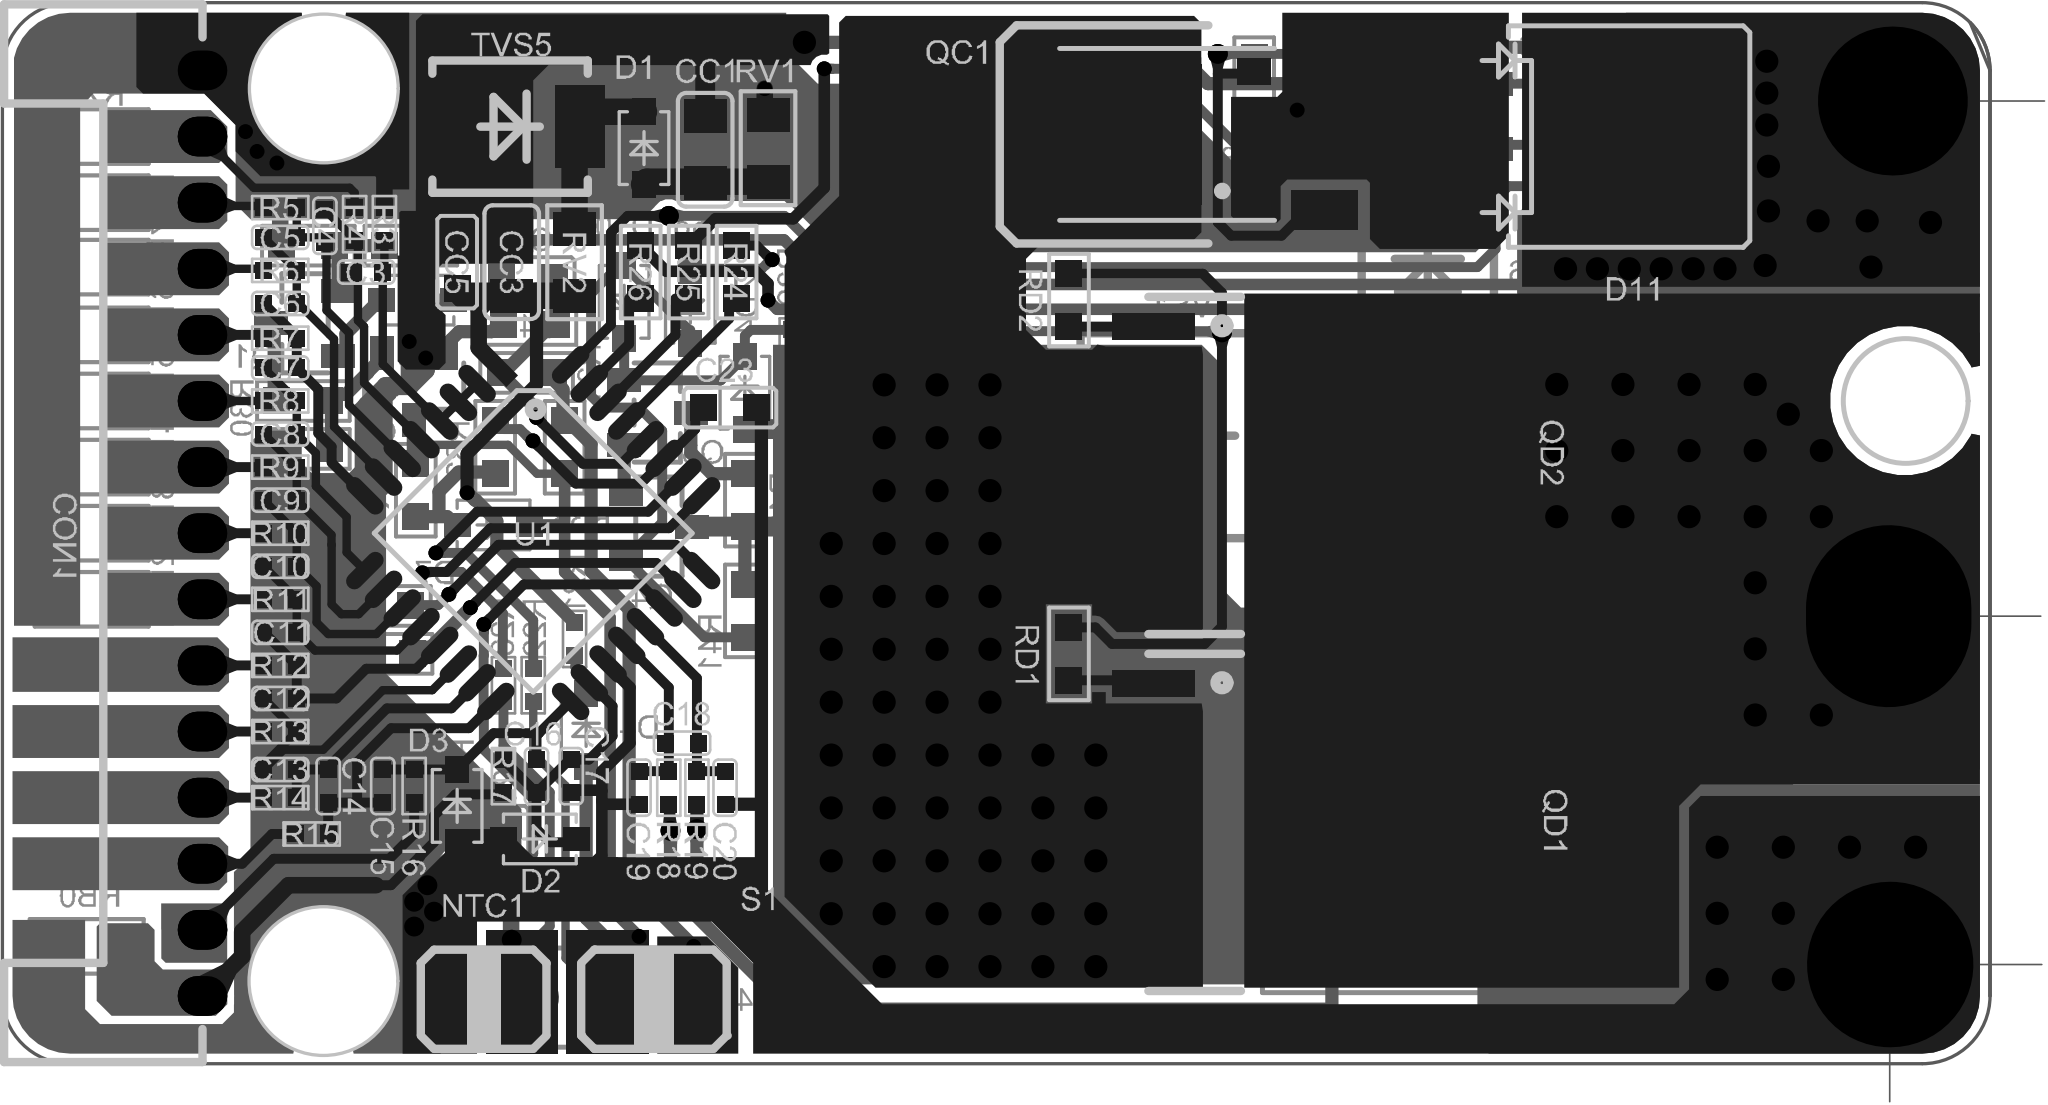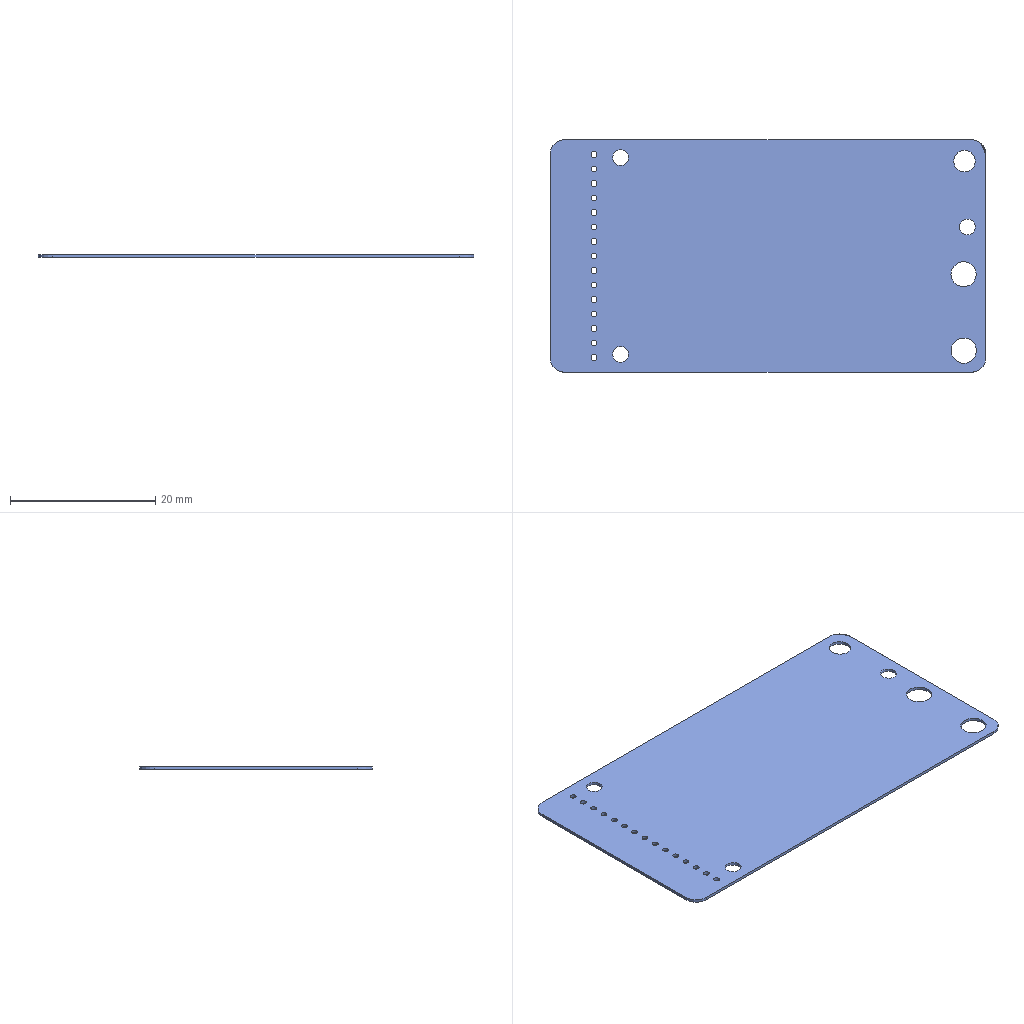Circuit board layout | Altium Designer | box 60.1 x 32.1 x 0.4 mm
Layer stack:
# Altium Designer layer stack of  (unit mm; dielectric type: 0 none, 1 core, 2 prepreg, 3 surface material)
index,name,kind,layer,copper_thickness_mm,dielectric_type,dielectric_thickness_mm,dielectric_material,dielectric_constant
0,Top Paste,other,,,,,,
1,Top Overlay,other,,,,,,
2,Top Solder,dielectric,,,3,0.0102,Solder Resist,3.5
3,Top Layer,copper,Top Layer,0.0356,,,,
4,Dielectric 1,dielectric,,,0,0.32,FR-4,4.8
5,Bottom Layer,copper,Bottom Layer,0.0356,,,,
6,Bottom Solder,dielectric,,,3,0.0102,Solder Resist,3.5
7,Bottom Overlay,other,,,,,,
8,Bottom Paste,other,,,,,,
# drill layer pairs: low layer,high layer
drill_pair,Top Layer,Bottom Layer
Part placement:
Designator,Comment,Layer,Footprint,Center-X(mm),Center-Y(mm),Rotation
D7,1N4148SW,BottomLayer,SOD323,14.8,0.25,180
ZD4,15V,BottomLayer,SOD323(1+2-),22.4,4.25,270
C1,0.1uF,BottomLayer,C0603A,15.85,7.75,180
QC1,NMOS,TopLayer,TO-252-DFN,35.416,12.065,0
RS3,R005,BottomLayer,R2512L,42.4,-12.05,180
RS2,R005,BottomLayer,R2512L,42.4,-7.95,180
RS1,R005,BottomLayer,R2512L,42.4,-3.85,180
TVS5,SMBJ64A,TopLayer,SMB_M(1+2-),15.3,12.3,180
D1,BAV21W,TopLayer,SOD323(1+2-),19.35,11.65,270
RX8,0Ω,BottomLayer,R0805L,2.65,12,0
RX7,0Ω,BottomLayer,R0805L,2.65,10,0
RX6,0Ω,BottomLayer,R0805L,2.65,8.05,0
RX5,0Ω,BottomLayer,R0805L,2.65,6,0
RX4,0Ω,BottomLayer,R0805L,2.65,4,0
RX3,0Ω,BottomLayer,R0805L,2.65,2,0
RX2,0Ω,BottomLayer,R0805L,2.65,0,0
RX1,0Ω,BottomLayer,R0805L,2.65,-2,0
RV2,100Ω,TopLayer,R0805L,17.25,8.2,90
RV1,1KΩ,TopLayer,R0805L,23.1,11.65,90
CC5,100nF/100V,TopLayer,C0603A,13.7,8.2,270
CC3,1uF/100V,TopLayer,C0805L,15.35,8.2,270
CC1,1uF/100V,TopLayer,C0805L,21.2,11.6,270
J4,UART,BottomLayer,CH-2.0-4P,17,-14.05,180
D2,BAT46WS,TopLayer,SOD323(1+2-),16.2,-9.25,180
NTC1,10KNTC,TopLayer,RT2.3X1-2,14.5,-14.1,180
D11,MBR10100DCT,TopLayer,TO-252-DIODE-DUAL,46.388,12,270
S1,SW-SPST,TopLayer,RT2.3X1.2-2,19.65,-14.1,0
RX,0R,BottomLayer,R0603A,12.45,1.3,270
R45,10M,BottomLayer,R0603A,15.9,6.3,180
R34,100K,BottomLayer,R0603A,15.8,4.85,180
R33,0Ω/NC,BottomLayer,R0603A,16.95,2.6,270
R32,100K,BottomLayer,R0603A,14.85,2.6,270
R31,100K,BottomLayer,R0603A,9.05,2.55,0
R30,1M,BottomLayer,R0603A,9.05,4,180
R29,100K,BottomLayer,R0603A,12.3,8.7,180
R28,20K,BottomLayer,R0603A,9.2,8.7,180
Q2,MMBT5551,BottomLayer,SOT23-3_BEC,12.4,4.442,0
Q1,MMBT5401,BottomLayer,SOT23-3_BEC,9.092,6.35,270
C14,0.1uF,TopLayer,C0402A,9.8,-7.65,90
R9,510R,TopLayer,R0402A,8.35,2,180
R8,510R,TopLayer,R0402A,8.35,4,180
R10,510R,TopLayer,R0402A,8.35,0,180
R13,510R,TopLayer,R0402A,8.35,-6,180
R12,510R,TopLayer,R0402A,8.35,-4,180
R11,510R,TopLayer,R0402A,8.35,-2,180
CON1,Header 15,TopLayer,PH-2.0mm15P弯脚不带扣,6,0,90
ZD2,15V,BottomLayer,SOD323(1+2-),12.5,7.05,180
ZD1,15V,BottomLayer,SOD323(1+2-),39.5,13.4,270
U1,SH3676016B,TopLayer,LQFP32L(PIN间距0.8mm),16,0,315
TVS1,75CA,BottomLayer,SMC,36.1,2.95,0
RTX,NC,BottomLayer,R0603A,13.8,-9.65,90
RT3,10K,BottomLayer,R0603A,11.5,-2.2,180
RT2,10K,BottomLayer,R0603A,11.55,-3.65,180
RD2,47R,TopLayer,R0603Ap,32.2,7.05,270
RD1,47R,TopLayer,R0603Ap,32.2,-3.65,270
RB0,51R,BottomLayer,R0805L,2.5,-12.5,0
R41,4.7M,BottomLayer,R0603A,22.4,-2.35,270
R40,510R,BottomLayer,R0603A,22.4,1,270
R39,10M,BottomLayer,R0402A,23.8,5.65,90
R38,1M,BottomLayer,R0603A,37.8,13.6,90
R37,3M,BottomLayer,R0603A,48.25,12.8,90
R36,1M,BottomLayer,R0603A,46.7,12.8,270
R27,3M,BottomLayer,R0603A,47.4,10.5,180
R26,1M,TopLayer,R0603A,19.25,7.9,270
R25,1K,TopLayer,R0603A,20.7,7.9,270
R24,1K,TopLayer,R0603A,22.15,7.9,270
R23,100R,BottomLayer,R0402A,15.1,-4.6,90
R22,100R,BottomLayer,R0402A,16,-4.6,90
R21,100R,BottomLayer,R0402A,17.25,-3.2,90
R19,10R,TopLayer,R0402A,20.95,-7.7,270
R18,10R,TopLayer,R0402A,20.1,-7.7,270
R17,510R,TopLayer,R0402A,15.1,-7.35,270
R16,510R,TopLayer,R0402A,12.4,-7.65,270
R15,510R,TopLayer,R0402A,9.3,-9.1,0
R14,510R,TopLayer,R0402A,8.35,-8,180
R7,510R,TopLayer,R0402A,8.35,5.9,180
R6,510R,TopLayer,R0402A,8.35,7.95,180
R5,510R,TopLayer,R0402A,8.35,9.85,180
R4,510R,TopLayer,R0402A,10.6,9.35,90
R3,510R,TopLayer,R0402A,11.5,9.35,90
QD2,NMOS,TopLayer,TOLL,38.15,2.05,270
QD1,NMOS,TopLayer,TOLL,38.15,-8.75,270
Q5,MMBT5401,BottomLayer,SOT23-3,44.092,12.6,270
Q4,MMBT5401,BottomLayer,SOT23-3,19.808,0.2,90
Q3,MMBT5401,BottomLayer,SOT23-3,19.758,3.65,90
D10,BAV21WS,BottomLayer,SOD323(1+2-),18.75,7,90
D9,BAV21WS,BottomLayer,SOD323(1+2-),20.75,6.85,90
D6,RS3M,BottomLayer,SMB_M(1+2-),43.05,7.8,270
D5,BAV21WS,BottomLayer,SOD323(1+2-),41.4,13.4,270
D4,BAV21WS,BottomLayer,SOD323(1+2-),17.6,-5.95,270
D3,BAT46WS,TopLayer,SOD323(1+2-),13.7,-8.25,270
C23,1uF/25V,TopLayer,C0603A,21.95,3.8,180
C21,1000PF,BottomLayer,C0603A,15.25,-9.65,90
C20,1uF,TopLayer,C0402A,21.8,-7.7,270
C19,1uF,TopLayer,C0402A,19.2,-7.7,270
C18,1000PF,TopLayer,C0402A,20.5,-6.35,180
C17,1uF,TopLayer,C0402A,17.15,-7.35,90
C16,0.1uF,TopLayer,C0402A,16.1,-7.35,90
C15,0.1uF,TopLayer,C0402A,11.45,-7.65,270
C13,0.1uF,TopLayer,C0402A,8.35,-7.15,180
C12,0.1uF,TopLayer,C0402A,8.35,-5,0
C11,0.1uF,TopLayer,C0402A,8.35,-3,0
C10,0.1uF,TopLayer,C0402A,8.35,-1,0
C9,0.1uF,TopLayer,C0402A,8.35,1,0
C8,0.1uF,TopLayer,C0402A,8.35,3,0
C7,0.1uF,TopLayer,C0402A,8.35,5,0
C6,0.1uF,TopLayer,C0402A,8.35,6.95,0
C5,0.1uF,TopLayer,C0402A,8.35,8.95,0
C4,0.1uF,TopLayer,C0402A,9.7,9.3,90
C3,0.1uF,TopLayer,C0402A,10.95,7.9,0
Pad and via stacks:
# Altium Designer via and pad stacks of  (unit mm). Each distinct definition once, with the count of objects using it.
# via: kind,start_layer,end_layer,hole_mm,diameter_mm,mode(0 simple;1 top-mid-bottom;2 full stack),diameter_per_layer,count,example_net
# pad: kind,layer,hole_mm,hole_type(0 round;1 square;2 slot),plating,top_size,top_shape(1 round;2 rect;3 octagon;9 rounded rect),mid_size,bottom_size,mode,footprint,size_per_layer,count,example
pad,Keep-Out Layer,0.025,0,plated,0.025x0.025,1,0.025x0.025,0.025x0.025,0,,,2,1
pad,Bottom Layer,0,0,plated,0.8x0.7,2,0.8x0.7,0.8x0.7,0,SOD323,,2,D7.2
pad,Bottom Layer,0,0,plated,0.8x0.8,2,0.8x0.8,0.8x0.8,0,R0603A,,36,R33.1
pad,Bottom Layer,0,0,plated,0.5x0.5,2,0.5x0.5,0.5x0.5,0,R0402A,,8,R39.2
pad,Bottom Layer,0,0,plated,2x3.2,2,2x3.2,2x3.2,0,R2512L,,6,RS2.1
pad,Bottom Layer,0,0,plated,1.016x1.27,2,1.016x1.27,1.016x1.27,0,R0805L,,18,RX8.1
pad,Bottom Layer,0,0,plated,0.8x0.7,2,0.8x0.7,0.8x0.7,0,SOD323(1+2-),,14,ZD4.1
pad,Bottom Layer,0,0,plated,0.8x0.8,2,0.8x0.8,0.8x0.8,0,C0603A,,4,C21.1
pad,Bottom Layer,0,0,plated,1.5x1.5,2,1.5x1.5,1.5x1.5,0,CH-2.0-4P,,1,J4.1
pad,Bottom Layer,0,0,plated,1.5x1.5,1,1.5x1.5,1.5x1.5,0,CH-2.0-4P,,3,J4.2
pad,Bottom Layer,0,0,plated,0.7x1,2,0.7x1,0.7x1,0,SOT23-3_BEC,,6,Q2.B
pad,Bottom Layer,0,0,plated,0.7x1,2,0.7x1,0.7x1,0,SOT23-3,,9,Q3.3
pad,Bottom Layer,0,0,plated,1.5x2.5,2,1.5x2.5,1.5x2.5,0,SMB M(1+2-),,2,D6.2
pad,Bottom Layer,0,0,plated,2.44x3.62,2,2.44x3.62,2.44x3.62,0,SMC,,2,TVS1.1
pad,Top Layer,0,0,plated,0.8x0.8,2,0.8x0.8,0.8x0.8,0,C0603A,,4,CC5.2
pad,Top Layer,0,0,plated,0.8x0.8,2,0.8x0.8,0.8x0.8,0,R0603A,,6,R24.2
pad,Top Layer,0,0,plated,0.5x0.5,2,0.5x0.5,0.5x0.5,0,C0402A,,36,C20.1
pad,Top Layer,0,0,plated,0.5x0.5,2,0.5x0.5,0.5x0.5,0,R0402A,,34,R19.2
pad,Top Layer,0,0,plated,2.5x0.8,2,2.5x0.8,2.5x0.8,0,TOLL,,2,QD2.1
pad,Top Layer,0,0,plated,1.7x0.8,2,1.7x0.8,1.7x0.8,0,TOLL,,14,QD2.2
pad,Top Layer,0,0,plated,0.8x8,2,0.8x8,0.8x8,0,TOLL,,2,QD2.2
pad,Top Layer,0,0,plated,9.9x8,2,9.9x8,9.9x8,0,TOLL,,2,QD2.3
pad,Top Layer,0,0,plated,3x4.26,2,3x4.26,3x4.26,0,TO-252-DFN,,1,QC1.3
pad,Top Layer,0,0,plated,1x0.8,2,1x0.8,1x0.8,0,TO-252-DFN,,8,QC1.2
pad,Top Layer,0,0,plated,1.2x2,2,1.2x2,1.2x2,0,TO-252-DFN,,2,QC1.1
pad,Top Layer,0,0,plated,5.3x1,2,5.3x1,5.3x1,0,TO-252-DFN,,1,QC1.3
pad,Top Layer,0,0,plated,6x6,2,6x6,6x6,0,TO-252-DIODE-DUAL,,1,D11.3
pad,Top Layer,0,0,plated,1.3x2.5,2,1.3x2.5,1.3x2.5,0,TO-252-DIODE-DUAL,,2,D11.2
pad,Top Layer,0,0,plated,0.8x0.8,2,0.8x0.8,0.8x0.8,0,R0603Ap,,4,RD1.1
pad,Top Layer,0,0,plated,1.016x1.27,2,1.016x1.27,1.016x1.27,0,R0805L,,4,RV2.2
pad,Top Layer,0,0,plated,1.5x2.5,2,1.5x2.5,1.5x2.5,0,SMB M(1+2-),,2,TVS5.2
pad,Top Layer,0,0,plated,1.016x1.27,2,1.016x1.27,1.016x1.27,0,C0805L,,4,CC1.1
pad,Top Layer,0,0,plated,1.2x2.3,1,1.2x2.3,1.2x2.3,0,RT2.3X1.2-2,,2,S1.1
pad,Top Layer,0,0,plated,1x2.3,1,1x2.3,1x2.3,0,RT2.3X1-2,,2,NTC1.1
pad,Top Layer,0,0,plated,0.8x0.7,2,0.8x0.7,0.8x0.7,0,SOD323(1+2-),,6,D2.1
pad,Top Layer,0,0,plated,0.5x1.4,1,0.5x1.4,0.5x1.4,0,LQFP32L(PIN\u00BC\u00E4\u00BE\u00E00.8mm),,31,U1.29
pad,Top Layer,0,0,plated,0.5x1.4,2,0.5x1.4,0.5x1.4,0,LQFP32L(PIN\u00BC\u00E4\u00BE\u00E00.8mm),,1,U1.1
pad,Multi-Layer,0.8,0,plated,1.5x1.2,1,1.5x1.2,1.5x1.2,0,PH-2.0mm15P\u00CD\u00E4\u00BD\u00C5\u00B2\u00BB\u00B4\u00F8\u00BF\u00DB,,15,CON1.11
pad,Multi-Layer,3.5,0,plated,5x5.5,1,5x5.5,5x5.5,0,,,1,2
pad,Multi-Layer,3,0,plated,4.5x4.5,1,4.5x4.5,4.5x4.5,0,,,1,2
pad,Multi-Layer,3.5,0,plated,5x5,1,5x5,5x5,0,,,1,2
pad,Top Solder,0,0,plated,12x2.5,2,12x2.5,12x2.5,0,,,1,2
pad,Top Solder,0,0,plated,20x2.5,2,20x2.5,20x2.5,0,,,1,2
pad,Top Solder,0,0,plated,15x2.5,2,15x2.5,15x2.5,0,,,2,2
pad,Bottom Solder,0,0,plated,15x2.5,2,15x2.5,15x2.5,0,,,2,2
via,Top Layer,Bottom Layer,0.3,0.45,0,,20,VCC1
via,Top Layer,Bottom Layer,0.4,0.6,0,,10,NetR27_2
via,Top Layer,Bottom Layer,0.5,0.7,0,,98,RS2
Copper pours:
name,layer,net,type(0 solid;1 hatched;2 none)
NONET_L-01_P-001,Bottom Layer,B+,0
RS2_L02_P042,Bottom Layer,RS2,0
P-_L02_P041,Bottom Layer,P-,0
NONET_L-01_P-001,Bottom Layer,B-,0
NONET_L-01_P-001,Bottom Layer,B0,0
NONET_L-01_P-001,Bottom Layer,B1,0
NONET_L-01_P-001,Bottom Layer,B2,0
NONET_L-01_P-001,Bottom Layer,B3,0
NONET_L-01_P-001,Bottom Layer,B4,0
NONET_L-01_P-001,Bottom Layer,B5,0
C-_L02_P032,Bottom Layer,C-,0
NONET_L-01_P-001,Bottom Layer,B12,0
NONET_L-01_P-001,Bottom Layer,B13,0
NONET_L-01_P-001,Bottom Layer,B6,0
NONET_L-01_P-001,Bottom Layer,B7,0
NONET_L-01_P-001,Bottom Layer,B8,0
NONET_L-01_P-001,Bottom Layer,B9,0
NONET_L-01_P-001,Bottom Layer,B10,0
NONET_L-01_P-001,Bottom Layer,B11,0
NONET_L-01_P-001,Bottom Layer,B-,0
RS2_L01_P029,Top Layer,RS2,0
NONET_L-01_P-001,Top Layer,B-,0
W,Top Layer,B-,0
B-_L01_P044,Top Layer,B-,0
C-_L01_P035,Top Layer,C-,0
B-_L01_P040,Top Layer,B-,0
NETC21_1_L01_P039,Top Layer,NetC21_1,0
NETD7_1_L01_P038,Top Layer,NetD7_1,0
NETR33_1_L01_P037,Top Layer,NetR33_1,0
B-_L01_P036,Top Layer,B-,0
P-_L01_P030,Top Layer,P-,0
NONET_L-01_P-001,Top Layer,B+,0
NONET_L-01_P-001,Top Layer,NetD11_1,0
Design rules, without the lines most boards share:
# Altium Designer design rules of  (exported by Altium Designer, unit mm)
# columns: name | kind | enabled | priority | scope1 | scope2 | descriptor | typed fields (field=value)
Schematic Supply Nets_1 | 41 | enabled | 1 | InNet('B-') | All | Supply Net(s)(InNet('B-')) |
Schematic Supply Nets | 41 | enabled | 2 | InNet('VCC1') | All | Supply Net(s)(InNet('VCC1')) |
NetAntennae | 56 | enabled | 1 | All | All | Net Antennae (Tolerance=0mm) (All) |
SilkToSilkClearance | 55 | enabled | 1 | All | All | Silk to Silk (Clearance=0mm) (All),(All) |
SilkToSolderMaskClearance | 54 | enabled | 1 | IsPad | All | Silk To Solder Mask (Clearance=0mm) (IsPad),(All) |
MinimumSolderMaskSliver | 53 | enabled | 1 | All | All | Minimum Solder Mask Sliver (Gap=0mm) (All),(All) |
HoleToHoleClearance | 52 | enabled | 1 | All | All | Hole To Hole Clearance (Gap=0mm) (All),(All) | gap=0
DiffPairsRouting | 51 | enabled | 1 | All | All | Differential Pairs Uncoupled Length using the Gap Constraints (Min=0.254mm) (Max=0.254mm) (Prefered=0.254mm)  and Width Constraints (Min=0.381mm) (Max=0.381mm) (Prefered=0.381mm) (All) |
HoleSize | 42 | enabled | 1 | All | All | Hole Size Constraint (Min=0.025mm) (Max=50mm) (All) |
Height | 50 | enabled | 1 | All | All | Height Constraint (Min=0mm) (Max=25.4mm) (Prefered=12.7mm) (All) | min_height=0 max_height=25.4
ComponentClearance | 24 | enabled | 1 | All | All | Component Clearance Constraint ( Horizontal Gap = 0mm, Vertical Gap = 0mm ) (All),(All)  | gap=0
SolderMaskExpansion | 13 | enabled | 1 | All | All | Solder Mask Expansion (Expansion =0.102mm) (All) | expansion=0.1016
PasteMaskExpansion | 14 | enabled | 1 | All | All | Paste Mask Expansion (Expansion =0mm) (All) | expansion=0
RoutingVias | 11 | enabled | 1 | All | All | Routing Via (MinHoleWidth=0.3mm) (MaxHoleWidth=0.4mm) (PreferredHoleWidth=0.4mm) (MinWidth=0.45mm) (MaxWidth=0.6mm) (PreferedWidth=0.6mm) (All) | via_min_hole=0.3 via_max_hole=0.4 via_preferred_diameter=0.6 via_preferred_hole=0.4
RoutingCorners | 10 | enabled | 1 | All | All | Routing Corners (Style=45-Degree) (Min Setback=2.54mm) (Max Setback=2.54mm) (All) |
Width | 2 | enabled | 1 | All | All | Width Constraint (Min=0.254mm) (Max=2mm) (Preferred=0.254mm) (All) |
PolygonConnect | 20 | enabled | 1 | All | All | Polygon Connect Rule(Direct Connect )(Conductor Width=0.254mm) (Relief Angle=90 Angle) (Entries=4) (Air Gap Width=0.254mm) (All),(All) | connect_style(0=relief,1=direct,2=none)=1 relief_conductor_width=0.254 relief_entries=4
PlaneClearance | 12 | enabled | 1 | All | All | Power Plane Clearance (Clearance =0.508mm) (All) | clearance=0.508
PlaneConnect | 6 | enabled | 1 | All | All | Power Plane Connect Rule(Direct Connect )(Expansion=0.508mm) (Conductor Width=0.254mm) (Air Gap=0.254mm) (Entries=4) (All) | relief_conductor_width=0.254 relief_entries=4 relief_expansion=0.508
Clearance | 0 | enabled | 1 | All | All | Clearance Constraint (Gap=0.2mm) (All),(All) | gap=0.2